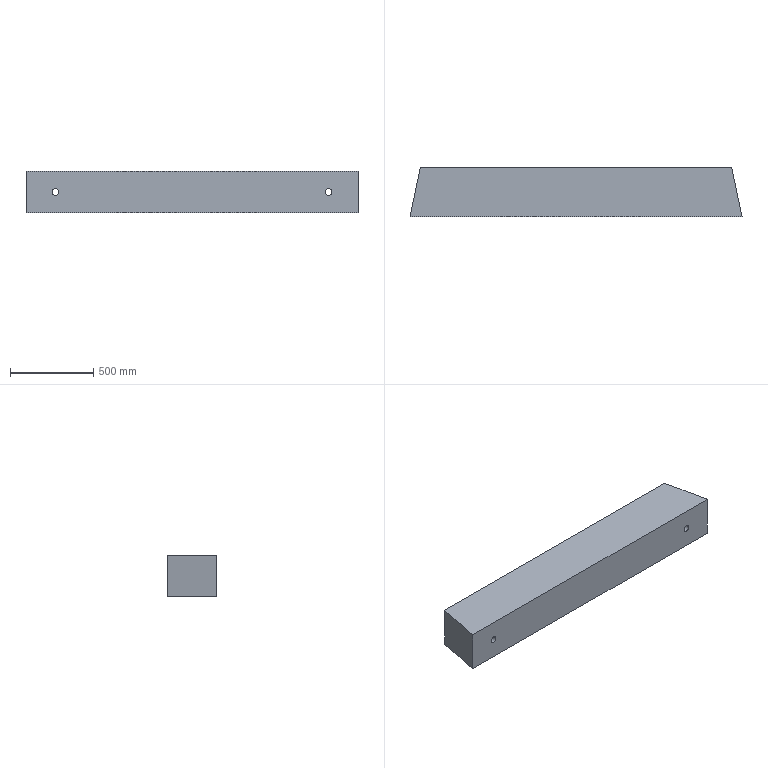Part | NX | features BREP 1 | 1 solid | 10 faces | box 2000 x 300 x 250 mm | volume 144558518 mm3 | plane 6 | cylinder 4 | commonest cylinder face diameters 40 x4
STEP:
#1=CARTESIAN_POINT('',(1298.,0.,0.));
#2=VERTEX_POINT('',#1);
#3=CARTESIAN_POINT('',(1258.,0.,0.));
#4=VERTEX_POINT('',#3);
#5=CARTESIAN_POINT('',(1278.,0.,0.));
#6=DIRECTION('',(0.,1.,0.));
#7=DIRECTION('',(1.,0.,0.));
#8=AXIS2_PLACEMENT_3D('',#5,#6,#7);
#9=CIRCLE('',#8,20.);
#10=EDGE_CURVE('',#2,#4,#9,.T.);
#11=ORIENTED_EDGE('',*,*,#10,.F.);
#12=CARTESIAN_POINT('',(1298.,300.,0.));
#13=VERTEX_POINT('',#12);
#14=CARTESIAN_POINT('',(1298.,0.,0.));
#15=DIRECTION('',(0.,1.,0.));
#16=VECTOR('',#15,1000.);
#17=LINE('',#14,#16);
#18=EDGE_CURVE('',#13,#2,#17,.F.);
#19=ORIENTED_EDGE('',*,*,#18,.F.);
#20=CARTESIAN_POINT('',(1258.,300.,0.));
#21=VERTEX_POINT('',#20);
#22=CARTESIAN_POINT('',(1278.,300.,0.));
#23=DIRECTION('',(0.,1.,0.));
#24=DIRECTION('',(1.,0.,0.));
#25=AXIS2_PLACEMENT_3D('',#22,#23,#24);
#26=CIRCLE('',#25,20.);
#27=EDGE_CURVE('',#13,#21,#26,.T.);
#28=ORIENTED_EDGE('',*,*,#27,.T.);
#29=CARTESIAN_POINT('',(1258.,0.,0.));
#30=DIRECTION('',(0.,1.,0.));
#31=VECTOR('',#30,1000.);
#32=LINE('',#29,#31);
#33=EDGE_CURVE('',#21,#4,#32,.F.);
#34=ORIENTED_EDGE('',*,*,#33,.T.);
#35=EDGE_LOOP('',(#11,#19,#28,#34));
#36=FACE_BOUND('',#35,.T.);
#37=CARTESIAN_POINT('',(1278.,0.,0.));
#38=DIRECTION('',(0.,1.,0.));
#39=DIRECTION('',(1.,0.,0.));
#40=AXIS2_PLACEMENT_3D('',#37,#38,#39);
#41=CYLINDRICAL_SURFACE('',#40,20.);
#42=ADVANCED_FACE('',(#36),#41,.F.);
#43=CARTESIAN_POINT('',(-347.,0.,0.));
#44=VERTEX_POINT('',#43);
#45=CARTESIAN_POINT('',(-387.,0.,0.));
#46=VERTEX_POINT('',#45);
#47=CARTESIAN_POINT('',(-367.,0.,0.));
#48=DIRECTION('',(0.,1.,0.));
#49=DIRECTION('',(-1.,0.,0.));
#50=AXIS2_PLACEMENT_3D('',#47,#48,#49);
#51=CIRCLE('',#50,20.);
#52=EDGE_CURVE('',#44,#46,#51,.T.);
#53=ORIENTED_EDGE('',*,*,#52,.F.);
#54=CARTESIAN_POINT('',(-347.,300.,0.));
#55=VERTEX_POINT('',#54);
#56=CARTESIAN_POINT('',(-347.,0.,0.));
#57=DIRECTION('',(0.,1.,0.));
#58=VECTOR('',#57,1000.);
#59=LINE('',#56,#58);
#60=EDGE_CURVE('',#55,#44,#59,.F.);
#61=ORIENTED_EDGE('',*,*,#60,.F.);
#62=CARTESIAN_POINT('',(-387.,300.,0.));
#63=VERTEX_POINT('',#62);
#64=CARTESIAN_POINT('',(-367.,300.,0.));
#65=DIRECTION('',(0.,1.,0.));
#66=DIRECTION('',(-1.,0.,0.));
#67=AXIS2_PLACEMENT_3D('',#64,#65,#66);
#68=CIRCLE('',#67,20.);
#69=EDGE_CURVE('',#55,#63,#68,.T.);
#70=ORIENTED_EDGE('',*,*,#69,.T.);
#71=CARTESIAN_POINT('',(-387.,0.,0.));
#72=DIRECTION('',(0.,1.,0.));
#73=VECTOR('',#72,1000.);
#74=LINE('',#71,#73);
#75=EDGE_CURVE('',#63,#46,#74,.F.);
#76=ORIENTED_EDGE('',*,*,#75,.T.);
#77=EDGE_LOOP('',(#53,#61,#70,#76));
#78=FACE_BOUND('',#77,.T.);
#79=CARTESIAN_POINT('',(-367.,0.,0.));
#80=DIRECTION('',(0.,1.,0.));
#81=DIRECTION('',(1.,0.,0.));
#82=AXIS2_PLACEMENT_3D('',#79,#80,#81);
#83=CYLINDRICAL_SURFACE('',#82,20.);
#84=ADVANCED_FACE('',(#78),#83,.F.);
#85=CARTESIAN_POINT('',(1455.5,0.,-125.));
#86=VERTEX_POINT('',#85);
#87=CARTESIAN_POINT('',(1393.,300.,-125.));
#88=VERTEX_POINT('',#87);
#89=CARTESIAN_POINT('',(1393.,300.,-125.));
#90=DIRECTION('',(-0.204,0.979,0.));
#91=VECTOR('',#90,1000.);
#92=LINE('',#89,#91);
#93=EDGE_CURVE('',#86,#88,#92,.T.);
#94=ORIENTED_EDGE('',*,*,#93,.T.);
#95=CARTESIAN_POINT('',(1393.,300.,125.));
#96=VERTEX_POINT('',#95);
#97=CARTESIAN_POINT('',(1393.,300.,125.));
#98=DIRECTION('',(0.,0.,-1.));
#99=VECTOR('',#98,1000.);
#100=LINE('',#97,#99);
#101=EDGE_CURVE('',#96,#88,#100,.T.);
#102=ORIENTED_EDGE('',*,*,#101,.F.);
#103=CARTESIAN_POINT('',(1455.5,0.,125.));
#104=VERTEX_POINT('',#103);
#105=CARTESIAN_POINT('',(1393.,300.,125.));
#106=DIRECTION('',(-0.204,0.979,0.));
#107=VECTOR('',#106,1000.);
#108=LINE('',#105,#107);
#109=EDGE_CURVE('',#104,#96,#108,.T.);
#110=ORIENTED_EDGE('',*,*,#109,.F.);
#111=CARTESIAN_POINT('',(1455.5,0.,125.));
#112=DIRECTION('',(0.,0.,-1.));
#113=VECTOR('',#112,1000.);
#114=LINE('',#111,#113);
#115=EDGE_CURVE('',#104,#86,#114,.T.);
#116=ORIENTED_EDGE('',*,*,#115,.T.);
#117=EDGE_LOOP('',(#94,#102,#110,#116));
#118=FACE_BOUND('',#117,.T.);
#119=CARTESIAN_POINT('',(1393.,300.,125.));
#120=DIRECTION('',(-0.979,-0.204,0.));
#121=DIRECTION('',(-0.204,0.979,0.));
#122=AXIS2_PLACEMENT_3D('',#119,#120,#121);
#123=PLANE('',#122);
#124=ADVANCED_FACE('',(#118),#123,.F.);
#125=CARTESIAN_POINT('',(1278.,300.,0.));
#126=DIRECTION('',(0.,1.,0.));
#127=DIRECTION('',(1.,0.,0.));
#128=AXIS2_PLACEMENT_3D('',#125,#126,#127);
#129=CIRCLE('',#128,20.);
#130=EDGE_CURVE('',#21,#13,#129,.T.);
#131=ORIENTED_EDGE('',*,*,#130,.F.);
#132=ORIENTED_EDGE('',*,*,#27,.F.);
#133=EDGE_LOOP('',(#131,#132));
#134=FACE_BOUND('',#133,.T.);
#135=CARTESIAN_POINT('',(-367.,300.,0.));
#136=DIRECTION('',(0.,1.,0.));
#137=DIRECTION('',(-1.,0.,0.));
#138=AXIS2_PLACEMENT_3D('',#135,#136,#137);
#139=CIRCLE('',#138,20.);
#140=EDGE_CURVE('',#63,#55,#139,.T.);
#141=ORIENTED_EDGE('',*,*,#140,.F.);
#142=ORIENTED_EDGE('',*,*,#69,.F.);
#143=EDGE_LOOP('',(#141,#142));
#144=FACE_BOUND('',#143,.T.);
#145=CARTESIAN_POINT('',(-482.,300.,-125.));
#146=VERTEX_POINT('',#145);
#147=CARTESIAN_POINT('',(-482.,300.,-125.));
#148=DIRECTION('',(-1.,0.,0.));
#149=VECTOR('',#148,1000.);
#150=LINE('',#147,#149);
#151=EDGE_CURVE('',#88,#146,#150,.T.);
#152=ORIENTED_EDGE('',*,*,#151,.T.);
#153=CARTESIAN_POINT('',(-482.,300.,125.));
#154=VERTEX_POINT('',#153);
#155=CARTESIAN_POINT('',(-482.,300.,125.));
#156=DIRECTION('',(0.,0.,-1.));
#157=VECTOR('',#156,1000.);
#158=LINE('',#155,#157);
#159=EDGE_CURVE('',#154,#146,#158,.T.);
#160=ORIENTED_EDGE('',*,*,#159,.F.);
#161=CARTESIAN_POINT('',(-482.,300.,125.));
#162=DIRECTION('',(-1.,0.,0.));
#163=VECTOR('',#162,1000.);
#164=LINE('',#161,#163);
#165=EDGE_CURVE('',#96,#154,#164,.T.);
#166=ORIENTED_EDGE('',*,*,#165,.F.);
#167=ORIENTED_EDGE('',*,*,#101,.T.);
#168=EDGE_LOOP('',(#152,#160,#166,#167));
#169=FACE_BOUND('',#168,.T.);
#170=CARTESIAN_POINT('',(-482.,300.,125.));
#171=DIRECTION('',(0.,-1.,0.));
#172=DIRECTION('',(-1.,0.,0.));
#173=AXIS2_PLACEMENT_3D('',#170,#171,#172);
#174=PLANE('',#173);
#175=ADVANCED_FACE('',(#134,#144,#169),#174,.F.);
#176=CARTESIAN_POINT('',(-544.5,0.,-125.));
#177=VERTEX_POINT('',#176);
#178=CARTESIAN_POINT('',(-544.5,0.,-125.));
#179=DIRECTION('',(-0.204,-0.979,0.));
#180=VECTOR('',#179,1000.);
#181=LINE('',#178,#180);
#182=EDGE_CURVE('',#146,#177,#181,.T.);
#183=ORIENTED_EDGE('',*,*,#182,.T.);
#184=CARTESIAN_POINT('',(-544.5,0.,125.));
#185=VERTEX_POINT('',#184);
#186=CARTESIAN_POINT('',(-544.5,0.,125.));
#187=DIRECTION('',(0.,0.,-1.));
#188=VECTOR('',#187,1000.);
#189=LINE('',#186,#188);
#190=EDGE_CURVE('',#185,#177,#189,.T.);
#191=ORIENTED_EDGE('',*,*,#190,.F.);
#192=CARTESIAN_POINT('',(-544.5,0.,125.));
#193=DIRECTION('',(-0.204,-0.979,0.));
#194=VECTOR('',#193,1000.);
#195=LINE('',#192,#194);
#196=EDGE_CURVE('',#154,#185,#195,.T.);
#197=ORIENTED_EDGE('',*,*,#196,.F.);
#198=ORIENTED_EDGE('',*,*,#159,.T.);
#199=EDGE_LOOP('',(#183,#191,#197,#198));
#200=FACE_BOUND('',#199,.T.);
#201=CARTESIAN_POINT('',(-544.5,0.,125.));
#202=DIRECTION('',(0.979,-0.204,0.));
#203=DIRECTION('',(-0.204,-0.979,0.));
#204=AXIS2_PLACEMENT_3D('',#201,#202,#203);
#205=PLANE('',#204);
#206=ADVANCED_FACE('',(#200),#205,.F.);
#207=CARTESIAN_POINT('',(1278.,0.,0.));
#208=DIRECTION('',(0.,1.,0.));
#209=DIRECTION('',(1.,0.,0.));
#210=AXIS2_PLACEMENT_3D('',#207,#208,#209);
#211=CIRCLE('',#210,20.);
#212=EDGE_CURVE('',#4,#2,#211,.T.);
#213=ORIENTED_EDGE('',*,*,#212,.T.);
#214=ORIENTED_EDGE('',*,*,#10,.T.);
#215=EDGE_LOOP('',(#213,#214));
#216=FACE_BOUND('',#215,.T.);
#217=CARTESIAN_POINT('',(-367.,0.,0.));
#218=DIRECTION('',(0.,1.,0.));
#219=DIRECTION('',(-1.,0.,0.));
#220=AXIS2_PLACEMENT_3D('',#217,#218,#219);
#221=CIRCLE('',#220,20.);
#222=EDGE_CURVE('',#46,#44,#221,.T.);
#223=ORIENTED_EDGE('',*,*,#222,.T.);
#224=ORIENTED_EDGE('',*,*,#52,.T.);
#225=EDGE_LOOP('',(#223,#224));
#226=FACE_BOUND('',#225,.T.);
#227=CARTESIAN_POINT('',(0.,0.,-125.));
#228=DIRECTION('',(1.,0.,0.));
#229=VECTOR('',#228,1000.);
#230=LINE('',#227,#229);
#231=EDGE_CURVE('',#177,#86,#230,.T.);
#232=ORIENTED_EDGE('',*,*,#231,.T.);
#233=ORIENTED_EDGE('',*,*,#115,.F.);
#234=CARTESIAN_POINT('',(1455.5,0.,125.));
#235=DIRECTION('',(1.,0.,0.));
#236=VECTOR('',#235,1000.);
#237=LINE('',#234,#236);
#238=EDGE_CURVE('',#185,#104,#237,.T.);
#239=ORIENTED_EDGE('',*,*,#238,.F.);
#240=ORIENTED_EDGE('',*,*,#190,.T.);
#241=EDGE_LOOP('',(#232,#233,#239,#240));
#242=FACE_BOUND('',#241,.T.);
#243=CARTESIAN_POINT('',(0.,0.,125.));
#244=DIRECTION('',(0.,1.,0.));
#245=DIRECTION('',(1.,0.,0.));
#246=AXIS2_PLACEMENT_3D('',#243,#244,#245);
#247=PLANE('',#246);
#248=ADVANCED_FACE('',(#216,#226,#242),#247,.F.);
#249=ORIENTED_EDGE('',*,*,#238,.T.);
#250=ORIENTED_EDGE('',*,*,#109,.T.);
#251=ORIENTED_EDGE('',*,*,#165,.T.);
#252=ORIENTED_EDGE('',*,*,#196,.T.);
#253=EDGE_LOOP('',(#249,#250,#251,#252));
#254=FACE_BOUND('',#253,.T.);
#255=CARTESIAN_POINT('',(1455.5,0.,125.));
#256=DIRECTION('',(0.,0.,1.));
#257=DIRECTION('',(-1.,0.,0.));
#258=AXIS2_PLACEMENT_3D('',#255,#256,#257);
#259=PLANE('',#258);
#260=ADVANCED_FACE('',(#254),#259,.T.);
#261=ORIENTED_EDGE('',*,*,#93,.F.);
#262=ORIENTED_EDGE('',*,*,#231,.F.);
#263=ORIENTED_EDGE('',*,*,#182,.F.);
#264=ORIENTED_EDGE('',*,*,#151,.F.);
#265=EDGE_LOOP('',(#261,#262,#263,#264));
#266=FACE_BOUND('',#265,.T.);
#267=CARTESIAN_POINT('',(1455.5,0.,-125.));
#268=DIRECTION('',(0.,0.,1.));
#269=DIRECTION('',(-1.,0.,0.));
#270=AXIS2_PLACEMENT_3D('',#267,#268,#269);
#271=PLANE('',#270);
#272=ADVANCED_FACE('',(#266),#271,.F.);
#273=ORIENTED_EDGE('',*,*,#60,.T.);
#274=ORIENTED_EDGE('',*,*,#222,.F.);
#275=ORIENTED_EDGE('',*,*,#75,.F.);
#276=ORIENTED_EDGE('',*,*,#140,.T.);
#277=EDGE_LOOP('',(#273,#274,#275,#276));
#278=FACE_BOUND('',#277,.T.);
#279=CARTESIAN_POINT('',(-367.,0.,0.));
#280=DIRECTION('',(0.,1.,0.));
#281=DIRECTION('',(1.,0.,0.));
#282=AXIS2_PLACEMENT_3D('',#279,#280,#281);
#283=CYLINDRICAL_SURFACE('',#282,20.);
#284=ADVANCED_FACE('',(#278),#283,.F.);
#285=ORIENTED_EDGE('',*,*,#18,.T.);
#286=ORIENTED_EDGE('',*,*,#212,.F.);
#287=ORIENTED_EDGE('',*,*,#33,.F.);
#288=ORIENTED_EDGE('',*,*,#130,.T.);
#289=EDGE_LOOP('',(#285,#286,#287,#288));
#290=FACE_BOUND('',#289,.T.);
#291=CARTESIAN_POINT('',(1278.,0.,0.));
#292=DIRECTION('',(0.,1.,0.));
#293=DIRECTION('',(1.,0.,0.));
#294=AXIS2_PLACEMENT_3D('',#291,#292,#293);
#295=CYLINDRICAL_SURFACE('',#294,20.);
#296=ADVANCED_FACE('',(#290),#295,.F.);
#297=CLOSED_SHELL('',(#42,#84,#124,#175,#206,#248,#260,#272,#284,#296));
#298=MANIFOLD_SOLID_BREP('',#297);
#299=(LENGTH_UNIT()NAMED_UNIT(*)SI_UNIT(.MILLI.,.METRE.));
#300=UNCERTAINTY_MEASURE_WITH_UNIT(LENGTH_MEASURE(0.00001),#299,'','');
#301=(NAMED_UNIT(*)PLANE_ANGLE_UNIT()SI_UNIT($,.RADIAN.));
#302=(NAMED_UNIT(*)SI_UNIT($,.STERADIAN.)SOLID_ANGLE_UNIT());
#303=(GEOMETRIC_REPRESENTATION_CONTEXT(3)GLOBAL_UNCERTAINTY_ASSIGNED_CONTEXT((#300))GLOBAL_UNIT_ASSIGNED_CONTEXT((#299,#301,#302))REPRESENTATION_CONTEXT('',''));
#304=ADVANCED_BREP_SHAPE_REPRESENTATION('',(#298),#303);